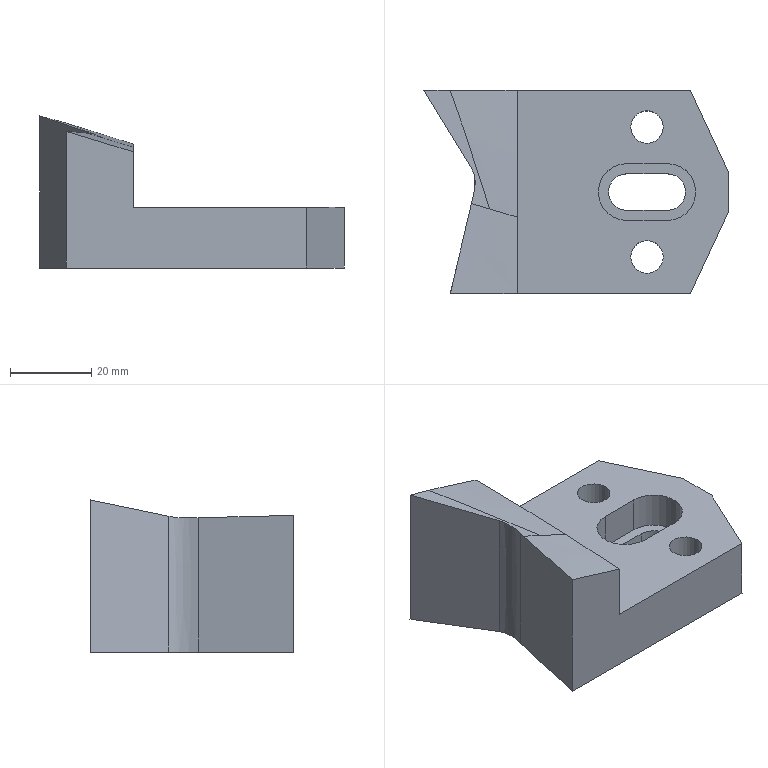Part | NX | features solid 2 | 1 solid | 25 faces | box 75.01 x 50.001 x 37.465 mm | volume 54539 mm3 | plane 13 | cylinder 6 | spline 6 | commonest cylinder face diameters 8 x2 9 x2 14 x2
STEP:
#1=CARTESIAN_POINT('',(745.,-33.,-80.));
#2=VERTEX_POINT('',#1);
#3=CARTESIAN_POINT('',(745.,-33.,-89.));
#4=VERTEX_POINT('',#3);
#5=CARTESIAN_POINT('',(745.,-33.,-90.));
#6=DIRECTION('',(0.000000502,-0.000000149,-1.));
#7=VECTOR('',#6,1000.);
#8=LINE('',#5,#7);
#9=EDGE_CURVE('',#2,#4,#8,.T.);
#10=ORIENTED_EDGE('',*,*,#9,.T.);
#11=CARTESIAN_POINT('',(745.,-47.,-89.));
#12=VERTEX_POINT('',#11);
#13=CARTESIAN_POINT('',(745.,-40.,-89.));
#14=DIRECTION('',(0.000000502,-0.000000149,-1.));
#15=DIRECTION('',(1.,0.,0.000000502));
#16=AXIS2_PLACEMENT_3D('',#13,#14,#15);
#17=CIRCLE('',#16,7.);
#18=EDGE_CURVE('',#4,#12,#17,.T.);
#19=ORIENTED_EDGE('',*,*,#18,.T.);
#20=CARTESIAN_POINT('',(745.,-47.,-80.));
#21=VERTEX_POINT('',#20);
#22=CARTESIAN_POINT('',(745.,-47.,-90.));
#23=DIRECTION('',(-0.000000502,0.000000149,1.));
#24=VECTOR('',#23,1000.);
#25=LINE('',#22,#24);
#26=EDGE_CURVE('',#21,#12,#25,.F.);
#27=ORIENTED_EDGE('',*,*,#26,.F.);
#28=CARTESIAN_POINT('',(745.,-40.,-80.));
#29=DIRECTION('',(-0.000000502,0.000000149,1.));
#30=DIRECTION('',(1.,0.,0.000000502));
#31=AXIS2_PLACEMENT_3D('',#28,#29,#30);
#32=CIRCLE('',#31,7.);
#33=EDGE_CURVE('',#21,#2,#32,.T.);
#34=ORIENTED_EDGE('',*,*,#33,.T.);
#35=EDGE_LOOP('',(#10,#19,#27,#34));
#36=FACE_BOUND('',#35,.T.);
#37=CARTESIAN_POINT('',(745.,-40.,-90.));
#38=DIRECTION('',(0.000000502,-0.000000149,-1.));
#39=DIRECTION('',(0.000001668,-1.,0.000000149));
#40=AXIS2_PLACEMENT_3D('',#37,#38,#39);
#41=CYLINDRICAL_SURFACE('',#40,7.);
#42=ADVANCED_FACE('',(#36),#41,.F.);
#43=ORIENTED_EDGE('',*,*,#26,.T.);
#44=CARTESIAN_POINT('',(735.,-47.,-89.));
#45=VERTEX_POINT('',#44);
#46=CARTESIAN_POINT('',(745.,-47.,-89.));
#47=DIRECTION('',(-1.,-0.000001668,-0.000000502));
#48=VECTOR('',#47,1000.);
#49=LINE('',#46,#48);
#50=EDGE_CURVE('',#12,#45,#49,.T.);
#51=ORIENTED_EDGE('',*,*,#50,.T.);
#52=CARTESIAN_POINT('',(735.,-47.,-80.));
#53=VERTEX_POINT('',#52);
#54=CARTESIAN_POINT('',(735.,-47.,-90.));
#55=DIRECTION('',(0.000000502,-0.000000149,-1.));
#56=VECTOR('',#55,1000.);
#57=LINE('',#54,#56);
#58=EDGE_CURVE('',#53,#45,#57,.T.);
#59=ORIENTED_EDGE('',*,*,#58,.F.);
#60=CARTESIAN_POINT('',(735.,-47.,-80.));
#61=DIRECTION('',(1.,0.000001668,0.000000502));
#62=VECTOR('',#61,1000.);
#63=LINE('',#60,#62);
#64=EDGE_CURVE('',#53,#21,#63,.T.);
#65=ORIENTED_EDGE('',*,*,#64,.T.);
#66=EDGE_LOOP('',(#43,#51,#59,#65));
#67=FACE_BOUND('',#66,.T.);
#68=CARTESIAN_POINT('',(735.,-47.,-90.));
#69=DIRECTION('',(-0.000001668,1.,-0.000000149));
#70=DIRECTION('',(-1.,-0.000001668,-0.000000502));
#71=AXIS2_PLACEMENT_3D('',#68,#69,#70);
#72=PLANE('',#71);
#73=ADVANCED_FACE('',(#67),#72,.T.);
#74=CARTESIAN_POINT('',(735.,-33.,-89.));
#75=VERTEX_POINT('',#74);
#76=CARTESIAN_POINT('',(735.,-40.,-89.));
#77=DIRECTION('',(-0.000000502,0.000000149,1.));
#78=DIRECTION('',(1.,0.,0.000000502));
#79=AXIS2_PLACEMENT_3D('',#76,#77,#78);
#80=CIRCLE('',#79,7.);
#81=EDGE_CURVE('',#75,#45,#80,.T.);
#82=ORIENTED_EDGE('',*,*,#81,.F.);
#83=CARTESIAN_POINT('',(735.,-33.,-80.));
#84=VERTEX_POINT('',#83);
#85=CARTESIAN_POINT('',(735.,-33.,-90.));
#86=DIRECTION('',(-0.000000502,0.000000149,1.));
#87=VECTOR('',#86,1000.);
#88=LINE('',#85,#87);
#89=EDGE_CURVE('',#84,#75,#88,.F.);
#90=ORIENTED_EDGE('',*,*,#89,.F.);
#91=CARTESIAN_POINT('',(735.,-40.,-80.));
#92=DIRECTION('',(-0.000000502,0.000000149,1.));
#93=DIRECTION('',(1.,0.,0.000000502));
#94=AXIS2_PLACEMENT_3D('',#91,#92,#93);
#95=CIRCLE('',#94,7.);
#96=EDGE_CURVE('',#53,#84,#95,.F.);
#97=ORIENTED_EDGE('',*,*,#96,.F.);
#98=ORIENTED_EDGE('',*,*,#58,.T.);
#99=EDGE_LOOP('',(#82,#90,#97,#98));
#100=FACE_BOUND('',#99,.T.);
#101=CARTESIAN_POINT('',(735.,-40.,-90.));
#102=DIRECTION('',(0.000000502,-0.000000149,-1.));
#103=DIRECTION('',(0.000001668,-1.,0.000000149));
#104=AXIS2_PLACEMENT_3D('',#101,#102,#103);
#105=CYLINDRICAL_SURFACE('',#104,7.);
#106=ADVANCED_FACE('',(#100),#105,.F.);
#107=CARTESIAN_POINT('',(745.,-33.,-89.));
#108=DIRECTION('',(-1.,-0.000001668,-0.000000502));
#109=VECTOR('',#108,1000.);
#110=LINE('',#107,#109);
#111=EDGE_CURVE('',#4,#75,#110,.T.);
#112=ORIENTED_EDGE('',*,*,#111,.F.);
#113=ORIENTED_EDGE('',*,*,#9,.F.);
#114=CARTESIAN_POINT('',(735.,-33.,-80.));
#115=DIRECTION('',(1.,0.000001668,0.000000502));
#116=VECTOR('',#115,1000.);
#117=LINE('',#114,#116);
#118=EDGE_CURVE('',#84,#2,#117,.T.);
#119=ORIENTED_EDGE('',*,*,#118,.F.);
#120=ORIENTED_EDGE('',*,*,#89,.T.);
#121=EDGE_LOOP('',(#112,#113,#119,#120));
#122=FACE_BOUND('',#121,.T.);
#123=CARTESIAN_POINT('',(735.,-33.,-90.));
#124=DIRECTION('',(-0.000001668,1.,-0.000000149));
#125=DIRECTION('',(-1.,-0.000001668,-0.000000502));
#126=AXIS2_PLACEMENT_3D('',#123,#124,#125);
#127=PLANE('',#126);
#128=ADVANCED_FACE('',(#122),#127,.F.);
#129=CARTESIAN_POINT('',(684.99,-15.,-95.));
#130=VERTEX_POINT('',#129);
#131=CARTESIAN_POINT('',(750.674,-15.,-95.));
#132=VERTEX_POINT('',#131);
#133=CARTESIAN_POINT('',(708.,-15.,-95.));
#134=DIRECTION('',(1.,0.000001668,0.000000502));
#135=VECTOR('',#134,1000.);
#136=LINE('',#133,#135);
#137=EDGE_CURVE('',#130,#132,#136,.T.);
#138=ORIENTED_EDGE('',*,*,#137,.T.);
#139=CARTESIAN_POINT('',(760.,-35.,-95.));
#140=VERTEX_POINT('',#139);
#141=CARTESIAN_POINT('',(750.674,-15.,-95.));
#142=DIRECTION('',(0.4226,-0.9063,0.000000347));
#143=VECTOR('',#142,1000.);
#144=LINE('',#141,#143);
#145=EDGE_CURVE('',#132,#140,#144,.T.);
#146=ORIENTED_EDGE('',*,*,#145,.T.);
#147=CARTESIAN_POINT('',(760.,-45.,-95.));
#148=VERTEX_POINT('',#147);
#149=CARTESIAN_POINT('',(760.,-45.,-95.));
#150=DIRECTION('',(-0.000001668,1.,-0.000000149));
#151=VECTOR('',#150,1000.);
#152=LINE('',#149,#151);
#153=EDGE_CURVE('',#148,#140,#152,.T.);
#154=ORIENTED_EDGE('',*,*,#153,.F.);
#155=CARTESIAN_POINT('',(750.674,-65.,-95.));
#156=VERTEX_POINT('',#155);
#157=CARTESIAN_POINT('',(750.674,-65.,-95.));
#158=DIRECTION('',(0.4226,0.9063,0.000000077));
#159=VECTOR('',#158,1000.);
#160=LINE('',#157,#159);
#161=EDGE_CURVE('',#156,#148,#160,.T.);
#162=ORIENTED_EDGE('',*,*,#161,.F.);
#163=CARTESIAN_POINT('',(691.52,-65.,-95.));
#164=VERTEX_POINT('',#163);
#165=CARTESIAN_POINT('',(700.,-65.,-95.));
#166=DIRECTION('',(1.,0.000001668,0.000000502));
#167=VECTOR('',#166,1000.);
#168=LINE('',#165,#167);
#169=EDGE_CURVE('',#164,#156,#168,.T.);
#170=ORIENTED_EDGE('',*,*,#169,.F.);
#171=CARTESIAN_POINT('',(697.072,-41.482,-95.));
#172=VERTEX_POINT('',#171);
#173=CARTESIAN_POINT('',(697.072,-41.482,-95.));
#174=CARTESIAN_POINT('',(695.176,-49.311,-95.));
#175=CARTESIAN_POINT('',(693.322,-57.15,-95.));
#176=CARTESIAN_POINT('',(691.52,-65.,-95.));
#177=B_SPLINE_CURVE_WITH_KNOTS('',3,(#173,#174,#175,#176),.UNSPECIFIED.,.F.,.F.,(4,4),(0.09346,0.1176),.UNSPECIFIED.);
#178=EDGE_CURVE('',#172,#164,#177,.T.);
#179=ORIENTED_EDGE('',*,*,#178,.F.);
#180=CARTESIAN_POINT('',(696.802,-34.28,-95.));
#181=VERTEX_POINT('',#180);
#182=CARTESIAN_POINT('',(696.802,-34.28,-95.));
#183=CARTESIAN_POINT('',(697.437,-35.339,-95.));
#184=CARTESIAN_POINT('',(697.892,-37.838,-95.));
#185=CARTESIAN_POINT('',(697.361,-40.28,-95.));
#186=CARTESIAN_POINT('',(697.072,-41.483,-95.));
#187=B_SPLINE_CURVE_WITH_KNOTS('',3,(#182,#183,#184,#185,#186),.UNSPECIFIED.,.F.,.F.,(4,1,4),(0.01374,0.01744,0.02115),.UNSPECIFIED.);
#188=EDGE_CURVE('',#172,#181,#187,.F.);
#189=ORIENTED_EDGE('',*,*,#188,.T.);
#190=CARTESIAN_POINT('',(684.99,-15.,-95.));
#191=CARTESIAN_POINT('',(688.941,-21.418,-95.));
#192=CARTESIAN_POINT('',(692.88,-27.844,-95.));
#193=CARTESIAN_POINT('',(696.802,-34.279,-95.));
#194=B_SPLINE_CURVE_WITH_KNOTS('',3,(#190,#191,#192,#193),.UNSPECIFIED.,.F.,.F.,(4,4),(0.,0.02261),.UNSPECIFIED.);
#195=EDGE_CURVE('',#130,#181,#194,.T.);
#196=ORIENTED_EDGE('',*,*,#195,.F.);
#197=EDGE_LOOP('',(#138,#146,#154,#162,#170,#179,#189,#196));
#198=FACE_BOUND('',#197,.T.);
#199=CARTESIAN_POINT('',(744.,-24.,-95.));
#200=VERTEX_POINT('',#199);
#201=CARTESIAN_POINT('',(740.,-24.,-95.));
#202=DIRECTION('',(-0.000000502,0.000000149,1.));
#203=DIRECTION('',(1.,0.,0.000000502));
#204=AXIS2_PLACEMENT_3D('',#201,#202,#203);
#205=CIRCLE('',#204,4.);
#206=EDGE_CURVE('',#200,#200,#205,.F.);
#207=ORIENTED_EDGE('',*,*,#206,.F.);
#208=EDGE_LOOP('',(#207));
#209=FACE_BOUND('',#208,.T.);
#210=CARTESIAN_POINT('',(744.,-56.,-95.));
#211=VERTEX_POINT('',#210);
#212=CARTESIAN_POINT('',(740.,-56.,-95.));
#213=DIRECTION('',(-0.000000502,0.000000149,1.));
#214=DIRECTION('',(1.,0.,0.000000502));
#215=AXIS2_PLACEMENT_3D('',#212,#213,#214);
#216=CIRCLE('',#215,4.);
#217=EDGE_CURVE('',#211,#211,#216,.F.);
#218=ORIENTED_EDGE('',*,*,#217,.F.);
#219=EDGE_LOOP('',(#218));
#220=FACE_BOUND('',#219,.T.);
#221=CARTESIAN_POINT('',(735.,-35.5,-95.));
#222=VERTEX_POINT('',#221);
#223=CARTESIAN_POINT('',(735.,-44.5,-95.));
#224=VERTEX_POINT('',#223);
#225=CARTESIAN_POINT('',(735.,-40.,-95.));
#226=DIRECTION('',(-0.000000502,0.000000149,1.));
#227=DIRECTION('',(1.,0.,0.000000502));
#228=AXIS2_PLACEMENT_3D('',#225,#226,#227);
#229=CIRCLE('',#228,4.5);
#230=EDGE_CURVE('',#222,#224,#229,.T.);
#231=ORIENTED_EDGE('',*,*,#230,.T.);
#232=CARTESIAN_POINT('',(745.,-44.5,-95.));
#233=VERTEX_POINT('',#232);
#234=CARTESIAN_POINT('',(735.,-44.5,-95.));
#235=DIRECTION('',(1.,0.000001668,0.000000502));
#236=VECTOR('',#235,1000.);
#237=LINE('',#234,#236);
#238=EDGE_CURVE('',#224,#233,#237,.T.);
#239=ORIENTED_EDGE('',*,*,#238,.T.);
#240=CARTESIAN_POINT('',(745.,-35.5,-95.));
#241=VERTEX_POINT('',#240);
#242=CARTESIAN_POINT('',(745.,-40.,-95.));
#243=DIRECTION('',(-0.000000502,0.000000149,1.));
#244=DIRECTION('',(1.,0.,0.000000502));
#245=AXIS2_PLACEMENT_3D('',#242,#243,#244);
#246=CIRCLE('',#245,4.5);
#247=EDGE_CURVE('',#233,#241,#246,.T.);
#248=ORIENTED_EDGE('',*,*,#247,.T.);
#249=CARTESIAN_POINT('',(735.,-35.5,-95.));
#250=DIRECTION('',(1.,0.000001668,0.000000502));
#251=VECTOR('',#250,1000.);
#252=LINE('',#249,#251);
#253=EDGE_CURVE('',#222,#241,#252,.T.);
#254=ORIENTED_EDGE('',*,*,#253,.F.);
#255=EDGE_LOOP('',(#231,#239,#248,#254));
#256=FACE_BOUND('',#255,.T.);
#257=CARTESIAN_POINT('',(700.,-15.,-95.));
#258=DIRECTION('',(0.000000502,-0.000000149,-1.));
#259=DIRECTION('',(0.000001668,-1.,0.000000149));
#260=AXIS2_PLACEMENT_3D('',#257,#258,#259);
#261=PLANE('',#260);
#262=ADVANCED_FACE('',(#198,#209,#220,#256),#261,.T.);
#263=CARTESIAN_POINT('',(691.497,-15.,-59.317));
#264=VERTEX_POINT('',#263);
#265=CARTESIAN_POINT('',(684.99,-15.,-57.535));
#266=VERTEX_POINT('',#265);
#267=CARTESIAN_POINT('',(691.486,-15.,-59.357));
#268=CARTESIAN_POINT('',(689.323,-15.,-58.741));
#269=CARTESIAN_POINT('',(687.16,-15.,-58.125));
#270=CARTESIAN_POINT('',(684.99,-15.,-57.535));
#271=B_SPLINE_CURVE_WITH_KNOTS('',3,(#267,#268,#269,#270),.UNSPECIFIED.,.F.,.F.,(4,4),(0.04155,0.0483),.UNSPECIFIED.);
#272=EDGE_CURVE('',#264,#266,#271,.T.);
#273=ORIENTED_EDGE('',*,*,#272,.F.);
#274=CARTESIAN_POINT('',(708.,-15.,-64.483));
#275=VERTEX_POINT('',#274);
#276=CARTESIAN_POINT('',(708.,-15.,-64.483));
#277=CARTESIAN_POINT('',(702.469,-15.,-62.856));
#278=CARTESIAN_POINT('',(697.041,-15.,-60.901));
#279=CARTESIAN_POINT('',(691.497,-15.,-59.317));
#280=B_SPLINE_CURVE_WITH_KNOTS('',3,(#276,#277,#278,#279),.UNSPECIFIED.,.F.,.F.,(4,4),(0.,0.01729),.UNSPECIFIED.);
#281=EDGE_CURVE('',#275,#264,#280,.T.);
#282=ORIENTED_EDGE('',*,*,#281,.F.);
#283=CARTESIAN_POINT('',(708.,-15.,-80.));
#284=VERTEX_POINT('',#283);
#285=CARTESIAN_POINT('',(708.,-15.,-105.));
#286=DIRECTION('',(-0.000000502,0.000000149,1.));
#287=VECTOR('',#286,1000.);
#288=LINE('',#285,#287);
#289=EDGE_CURVE('',#275,#284,#288,.F.);
#290=ORIENTED_EDGE('',*,*,#289,.T.);
#291=CARTESIAN_POINT('',(750.674,-15.,-80.));
#292=VERTEX_POINT('',#291);
#293=CARTESIAN_POINT('',(708.,-15.,-80.));
#294=DIRECTION('',(1.,0.000001668,0.000000502));
#295=VECTOR('',#294,1000.);
#296=LINE('',#293,#295);
#297=EDGE_CURVE('',#284,#292,#296,.T.);
#298=ORIENTED_EDGE('',*,*,#297,.T.);
#299=CARTESIAN_POINT('',(750.674,-15.,-90.));
#300=DIRECTION('',(0.000000502,-0.000000149,-1.));
#301=VECTOR('',#300,1000.);
#302=LINE('',#299,#301);
#303=EDGE_CURVE('',#292,#132,#302,.T.);
#304=ORIENTED_EDGE('',*,*,#303,.T.);
#305=ORIENTED_EDGE('',*,*,#137,.F.);
#306=CARTESIAN_POINT('',(684.99,-15.,-57.535));
#307=CARTESIAN_POINT('',(684.99,-15.,-70.023));
#308=CARTESIAN_POINT('',(684.99,-15.,-82.512));
#309=CARTESIAN_POINT('',(684.99,-15.,-95.));
#310=B_SPLINE_CURVE_WITH_KNOTS('',3,(#306,#307,#308,#309),.UNSPECIFIED.,.F.,.F.,(4,4),(0.00214,0.03961),.UNSPECIFIED.);
#311=EDGE_CURVE('',#266,#130,#310,.T.);
#312=ORIENTED_EDGE('',*,*,#311,.F.);
#313=EDGE_LOOP('',(#273,#282,#290,#298,#304,#305,#312));
#314=FACE_BOUND('',#313,.T.);
#315=CARTESIAN_POINT('',(708.,-15.,-90.));
#316=DIRECTION('',(-0.000001668,1.,-0.000000149));
#317=DIRECTION('',(-1.,-0.000001668,-0.000000502));
#318=AXIS2_PLACEMENT_3D('',#315,#316,#317);
#319=PLANE('',#318);
#320=ADVANCED_FACE('',(#314),#319,.T.);
#321=CARTESIAN_POINT('',(691.535,-65.,-61.337));
#322=VERTEX_POINT('',#321);
#323=CARTESIAN_POINT('',(691.535,-65.,-61.337));
#324=CARTESIAN_POINT('',(691.53,-65.,-72.558));
#325=CARTESIAN_POINT('',(691.525,-65.,-83.779));
#326=CARTESIAN_POINT('',(691.52,-65.,-95.));
#327=B_SPLINE_CURVE_WITH_KNOTS('',3,(#323,#324,#325,#326),.UNSPECIFIED.,.F.,.F.,(4,4),(0.002194,0.03586),.UNSPECIFIED.);
#328=EDGE_CURVE('',#322,#164,#327,.T.);
#329=ORIENTED_EDGE('',*,*,#328,.T.);
#330=ORIENTED_EDGE('',*,*,#169,.T.);
#331=CARTESIAN_POINT('',(750.674,-65.,-80.));
#332=VERTEX_POINT('',#331);
#333=CARTESIAN_POINT('',(750.674,-65.,-90.));
#334=DIRECTION('',(0.000000502,-0.000000149,-1.));
#335=VECTOR('',#334,1000.);
#336=LINE('',#333,#335);
#337=EDGE_CURVE('',#332,#156,#336,.T.);
#338=ORIENTED_EDGE('',*,*,#337,.F.);
#339=CARTESIAN_POINT('',(708.,-65.,-80.));
#340=VERTEX_POINT('',#339);
#341=CARTESIAN_POINT('',(700.,-65.,-80.));
#342=DIRECTION('',(1.,0.000001668,0.000000502));
#343=VECTOR('',#342,1000.);
#344=LINE('',#341,#343);
#345=EDGE_CURVE('',#340,#332,#344,.T.);
#346=ORIENTED_EDGE('',*,*,#345,.F.);
#347=CARTESIAN_POINT('',(708.,-65.,-66.363));
#348=VERTEX_POINT('',#347);
#349=CARTESIAN_POINT('',(708.,-65.,-105.));
#350=DIRECTION('',(-0.000000502,0.000000149,1.));
#351=VECTOR('',#350,1000.);
#352=LINE('',#349,#351);
#353=EDGE_CURVE('',#348,#340,#352,.F.);
#354=ORIENTED_EDGE('',*,*,#353,.F.);
#355=CARTESIAN_POINT('',(691.535,-65.,-61.337));
#356=CARTESIAN_POINT('',(697.046,-65.,-62.922));
#357=CARTESIAN_POINT('',(702.528,-65.,-64.628));
#358=CARTESIAN_POINT('',(708.,-65.,-66.363));
#359=B_SPLINE_CURVE_WITH_KNOTS('',3,(#355,#356,#357,#358),.UNSPECIFIED.,.F.,.F.,(4,4),(0.0434,0.0606),.UNSPECIFIED.);
#360=EDGE_CURVE('',#322,#348,#359,.T.);
#361=ORIENTED_EDGE('',*,*,#360,.F.);
#362=EDGE_LOOP('',(#329,#330,#338,#346,#354,#361));
#363=FACE_BOUND('',#362,.T.);
#364=CARTESIAN_POINT('',(700.,-65.,-90.));
#365=DIRECTION('',(-0.000001668,1.,-0.000000149));
#366=DIRECTION('',(0.000000502,-0.000000149,-1.));
#367=AXIS2_PLACEMENT_3D('',#364,#365,#366);
#368=PLANE('',#367);
#369=ADVANCED_FACE('',(#363),#368,.F.);
#370=CARTESIAN_POINT('',(696.733,-42.883,-61.871));
#371=VERTEX_POINT('',#370);
#372=CARTESIAN_POINT('',(696.733,-42.883,-61.871));
#373=CARTESIAN_POINT('',(694.956,-50.244,-61.658));
#374=CARTESIAN_POINT('',(693.223,-57.617,-61.47));
#375=CARTESIAN_POINT('',(691.535,-65.,-61.337));
#376=B_SPLINE_CURVE_WITH_KNOTS('',3,(#372,#373,#374,#375),.UNSPECIFIED.,.F.,.F.,(4,4),(0.1439,0.1667),.UNSPECIFIED.);
#377=EDGE_CURVE('',#371,#322,#376,.T.);
#378=ORIENTED_EDGE('',*,*,#377,.T.);
#379=ORIENTED_EDGE('',*,*,#360,.T.);
#380=CARTESIAN_POINT('',(708.,-46.209,-65.274));
#381=VERTEX_POINT('',#380);
#382=CARTESIAN_POINT('',(708.,-65.,-66.363));
#383=CARTESIAN_POINT('',(708.,-63.434,-66.267));
#384=CARTESIAN_POINT('',(708.,-61.092,-66.12));
#385=CARTESIAN_POINT('',(708.,-58.339,-65.945));
#386=CARTESIAN_POINT('',(708.,-56.795,-65.847));
#387=CARTESIAN_POINT('',(708.,-55.553,-65.766));
#388=CARTESIAN_POINT('',(708.,-54.635,-65.708));
#389=CARTESIAN_POINT('',(708.,-53.211,-65.623));
#390=CARTESIAN_POINT('',(708.,-50.605,-65.479));
#391=CARTESIAN_POINT('',(708.,-48.045,-65.356));
#392=CARTESIAN_POINT('',(708.,-46.209,-65.274));
#393=B_SPLINE_CURVE_WITH_KNOTS('',3,(#382,#383,#384,#385,#386,#387,#388,#389,#390,#391,#392),.UNSPECIFIED.,.F.,.F.,(4,1,1,1,1,1,1,1,4),(0.,0.25,0.375,0.4375,0.5,0.5625,0.625,0.75,1.),.UNSPECIFIED.);
#394=EDGE_CURVE('',#381,#348,#393,.F.);
#395=ORIENTED_EDGE('',*,*,#394,.F.);
#396=CARTESIAN_POINT('',(701.201,-44.201,-63.22));
#397=VERTEX_POINT('',#396);
#398=CARTESIAN_POINT('',(701.2,-44.202,-63.22));
#399=CARTESIAN_POINT('',(703.467,-44.871,-63.905));
#400=CARTESIAN_POINT('',(705.733,-45.54,-64.589));
#401=CARTESIAN_POINT('',(708.,-46.209,-65.274));
#402=B_SPLINE_CURVE_WITH_KNOTS('',3,(#398,#399,#400,#401),.UNSPECIFIED.,.F.,.F.,(4,4),(0.4767,0.7872),.UNSPECIFIED.);
#403=EDGE_CURVE('',#397,#381,#402,.T.);
#404=ORIENTED_EDGE('',*,*,#403,.F.);
#405=CARTESIAN_POINT('',(696.733,-42.883,-61.871));
#406=CARTESIAN_POINT('',(698.222,-43.323,-62.321));
#407=CARTESIAN_POINT('',(699.711,-43.762,-62.77));
#408=CARTESIAN_POINT('',(701.2,-44.202,-63.22));
#409=B_SPLINE_CURVE_WITH_KNOTS('',3,(#405,#406,#407,#408),.UNSPECIFIED.,.F.,.F.,(4,4),(0.2727,0.4767),.UNSPECIFIED.);
#410=EDGE_CURVE('',#371,#397,#409,.T.);
#411=ORIENTED_EDGE('',*,*,#410,.F.);
#412=EDGE_LOOP('',(#378,#379,#395,#404,#411));
#413=FACE_BOUND('',#412,.T.);
#414=CARTESIAN_POINT('',(707.217,-68.842,-66.332));
#415=CARTESIAN_POINT('',(708.034,-65.269,-66.411));
#416=CARTESIAN_POINT('',(709.678,-58.129,-66.434));
#417=CARTESIAN_POINT('',(711.425,-51.027,-66.483));
#418=CARTESIAN_POINT('',(712.345,-47.491,-66.586));
#419=CARTESIAN_POINT('',(701.97,-67.603,-64.574));
#420=CARTESIAN_POINT('',(702.795,-63.984,-64.655));
#421=CARTESIAN_POINT('',(704.448,-56.747,-64.764));
#422=CARTESIAN_POINT('',(706.192,-49.538,-64.898));
#423=CARTESIAN_POINT('',(707.11,-45.946,-65.005));
#424=CARTESIAN_POINT('',(696.701,-66.359,-62.886));
#425=CARTESIAN_POINT('',(697.536,-62.692,-62.963));
#426=CARTESIAN_POINT('',(699.208,-55.36,-63.123));
#427=CARTESIAN_POINT('',(700.959,-48.048,-63.314));
#428=CARTESIAN_POINT('',(701.875,-44.401,-63.424));
#429=CARTESIAN_POINT('',(691.402,-65.109,-61.304));
#430=CARTESIAN_POINT('',(692.251,-61.394,-61.371));
#431=CARTESIAN_POINT('',(693.957,-53.966,-61.527));
#432=CARTESIAN_POINT('',(695.727,-46.555,-61.73));
#433=CARTESIAN_POINT('',(696.64,-42.856,-61.843));
#434=B_SPLINE_SURFACE_WITH_KNOTS('',3,3,((#414,#415,#416,#417,#418),(#419,#420,#421,#422,#423),(#424,#425,#426,#427,#428),(#429,#430,#431,#432,#433)),.UNSPECIFIED.,.F.,.F.,.F.,(4,4),(4,1,4),(0.0881,0.7516),(0.04208,0.521,1.),.UNSPECIFIED.);
#435=ADVANCED_FACE('',(#413),#434,.F.);
#436=CARTESIAN_POINT('',(696.802,-34.279,-61.549));
#437=VERTEX_POINT('',#436);
#438=CARTESIAN_POINT('',(697.072,-41.482,-61.912));
#439=VERTEX_POINT('',#438);
#440=CARTESIAN_POINT('',(696.802,-34.279,-61.549));
#441=CARTESIAN_POINT('',(697.43,-35.326,-61.77));
#442=CARTESIAN_POINT('',(697.897,-37.829,-62.003));
#443=CARTESIAN_POINT('',(697.362,-40.276,-61.947));
#444=CARTESIAN_POINT('',(697.072,-41.483,-61.912));
#445=B_SPLINE_CURVE_WITH_KNOTS('',3,(#440,#441,#442,#443,#444),.UNSPECIFIED.,.F.,.F.,(4,1,4),(0.01176,0.01548,0.0192),.UNSPECIFIED.);
#446=EDGE_CURVE('',#437,#439,#445,.T.);
#447=ORIENTED_EDGE('',*,*,#446,.T.);
#448=CARTESIAN_POINT('',(696.733,-42.883,-61.871));
#449=CARTESIAN_POINT('',(696.846,-42.416,-61.885));
#450=CARTESIAN_POINT('',(696.959,-41.949,-61.898));
#451=CARTESIAN_POINT('',(697.072,-41.482,-61.912));
#452=B_SPLINE_CURVE_WITH_KNOTS('',3,(#448,#449,#450,#451),.UNSPECIFIED.,.F.,.F.,(4,4),(0.,0.001442),.UNSPECIFIED.);
#453=EDGE_CURVE('',#371,#439,#452,.T.);
#454=ORIENTED_EDGE('',*,*,#453,.F.);
#455=ORIENTED_EDGE('',*,*,#410,.T.);
#456=CARTESIAN_POINT('',(695.108,-25.285,-60.731));
#457=VERTEX_POINT('',#456);
#458=CARTESIAN_POINT('',(701.201,-44.2,-63.22));
#459=CARTESIAN_POINT('',(699.21,-38.,-62.382));
#460=CARTESIAN_POINT('',(697.18,-31.694,-61.551));
#461=CARTESIAN_POINT('',(695.109,-25.284,-60.732));
#462=B_SPLINE_CURVE_WITH_KNOTS('',3,(#458,#459,#460,#461),.UNSPECIFIED.,.F.,.F.,(4,4),(0.,0.2626),.UNSPECIFIED.);
#463=EDGE_CURVE('',#397,#457,#462,.T.);
#464=ORIENTED_EDGE('',*,*,#463,.T.);
#465=CARTESIAN_POINT('',(695.108,-25.284,-60.732));
#466=CARTESIAN_POINT('',(693.918,-21.621,-60.262));
#467=CARTESIAN_POINT('',(692.708,-18.186,-59.804));
#468=CARTESIAN_POINT('',(691.48,-14.985,-59.355));
#469=B_SPLINE_CURVE_WITH_KNOTS('',3,(#465,#466,#467,#468),.UNSPECIFIED.,.F.,.F.,(4,4),(0.01082,0.3147),.UNSPECIFIED.);
#470=EDGE_CURVE('',#457,#264,#469,.T.);
#471=ORIENTED_EDGE('',*,*,#470,.T.);
#472=ORIENTED_EDGE('',*,*,#272,.T.);
#473=CARTESIAN_POINT('',(696.802,-34.279,-61.549));
#474=CARTESIAN_POINT('',(692.883,-27.849,-60.173));
#475=CARTESIAN_POINT('',(688.946,-21.425,-58.809));
#476=CARTESIAN_POINT('',(684.99,-15.,-57.535));
#477=B_SPLINE_CURVE_WITH_KNOTS('',3,(#473,#474,#475,#476),.UNSPECIFIED.,.F.,.F.,(4,4),(0.1292,0.1521),.UNSPECIFIED.);
#478=EDGE_CURVE('',#437,#266,#477,.T.);
#479=ORIENTED_EDGE('',*,*,#478,.F.);
#480=EDGE_LOOP('',(#447,#454,#455,#464,#471,#472,#479));
#481=FACE_BOUND('',#480,.T.);
#482=CARTESIAN_POINT('',(701.297,-44.386,-63.256));
#483=CARTESIAN_POINT('',(696.609,-43.003,-61.851));
#484=CARTESIAN_POINT('',(691.903,-41.618,-60.391));
#485=CARTESIAN_POINT('',(687.233,-40.237,-59.041));
#486=CARTESIAN_POINT('',(700.592,-35.466,-62.673));
#487=CARTESIAN_POINT('',(695.858,-33.953,-61.261));
#488=CARTESIAN_POINT('',(691.106,-32.435,-59.794));
#489=CARTESIAN_POINT('',(686.391,-30.927,-58.438));
#490=CARTESIAN_POINT('',(699.871,-26.547,-62.126));
#491=CARTESIAN_POINT('',(695.091,-24.907,-60.71));
#492=CARTESIAN_POINT('',(690.294,-23.258,-59.239));
#493=CARTESIAN_POINT('',(685.532,-21.625,-57.879));
#494=CARTESIAN_POINT('',(699.134,-17.631,-61.617));
#495=CARTESIAN_POINT('',(694.308,-15.865,-60.199));
#496=CARTESIAN_POINT('',(689.465,-14.087,-58.725));
#497=CARTESIAN_POINT('',(684.657,-12.332,-57.363));
#498=B_SPLINE_SURFACE_WITH_KNOTS('',3,3,((#482,#483,#484,#485),(#486,#487,#488,#489),(#490,#491,#492,#493),(#494,#495,#496,#497)),.UNSPECIFIED.,.F.,.F.,.F.,(4,4),(4,4),(-0.0006687,0.1104),(0.1077,0.2017),.UNSPECIFIED.);
#499=ADVANCED_FACE('',(#481),#498,.T.);
#500=ORIENTED_EDGE('',*,*,#394,.T.);
#501=ORIENTED_EDGE('',*,*,#353,.T.);
#502=CARTESIAN_POINT('',(708.,-15.,-80.));
#503=DIRECTION('',(-0.000001668,1.,-0.000000149));
#504=VECTOR('',#503,1000.);
#505=LINE('',#502,#504);
#506=EDGE_CURVE('',#284,#340,#505,.F.);
#507=ORIENTED_EDGE('',*,*,#506,.F.);
#508=ORIENTED_EDGE('',*,*,#289,.F.);
#509=CARTESIAN_POINT('',(708.,-46.209,-65.274));
#510=CARTESIAN_POINT('',(708.,-36.298,-64.834));
#511=CARTESIAN_POINT('',(708.,-25.895,-64.57));
#512=CARTESIAN_POINT('',(708.,-15.,-64.483));
#513=B_SPLINE_CURVE_WITH_KNOTS('',3,(#509,#510,#511,#512),.UNSPECIFIED.,.F.,.F.,(4,4),(0.,1.),.UNSPECIFIED.);
#514=EDGE_CURVE('',#381,#275,#513,.T.);
#515=ORIENTED_EDGE('',*,*,#514,.F.);
#516=EDGE_LOOP('',(#500,#501,#507,#508,#515));
#517=FACE_BOUND('',#516,.T.);
#518=CARTESIAN_POINT('',(708.,-15.,-105.));
#519=DIRECTION('',(-1.,-0.000001668,-0.000000502));
#520=DIRECTION('',(0.000001668,-1.,0.000000149));
#521=AXIS2_PLACEMENT_3D('',#518,#519,#520);
#522=PLANE('',#521);
#523=ADVANCED_FACE('',(#517),#522,.F.);
#524=CARTESIAN_POINT('',(744.,-24.,-80.));
#525=VERTEX_POINT('',#524);
#526=CARTESIAN_POINT('',(740.,-24.,-80.));
#527=DIRECTION('',(-0.000000502,0.000000149,1.));
#528=DIRECTION('',(1.,0.,0.000000502));
#529=AXIS2_PLACEMENT_3D('',#526,#527,#528);
#530=CIRCLE('',#529,4.);
#531=EDGE_CURVE('',#525,#525,#530,.F.);
#532=ORIENTED_EDGE('',*,*,#531,.T.);
#533=EDGE_LOOP('',(#532));
#534=FACE_BOUND('',#533,.T.);
#535=CARTESIAN_POINT('',(744.,-56.,-80.));
#536=VERTEX_POINT('',#535);
#537=CARTESIAN_POINT('',(740.,-56.,-80.));
#538=DIRECTION('',(-0.000000502,0.000000149,1.));
#539=DIRECTION('',(1.,0.,0.000000502));
#540=AXIS2_PLACEMENT_3D('',#537,#538,#539);
#541=CIRCLE('',#540,4.);
#542=EDGE_CURVE('',#536,#536,#541,.F.);
#543=ORIENTED_EDGE('',*,*,#542,.T.);
#544=EDGE_LOOP('',(#543));
#545=FACE_BOUND('',#544,.T.);
#546=ORIENTED_EDGE('',*,*,#297,.F.);
#547=ORIENTED_EDGE('',*,*,#506,.T.);
#548=ORIENTED_EDGE('',*,*,#345,.T.);
#549=CARTESIAN_POINT('',(760.,-45.,-80.));
#550=VERTEX_POINT('',#549);
#551=CARTESIAN_POINT('',(750.674,-65.,-80.));
#552=DIRECTION('',(0.4226,0.9063,0.000000077));
#553=VECTOR('',#552,1000.);
#554=LINE('',#551,#553);
#555=EDGE_CURVE('',#332,#550,#554,.T.);
#556=ORIENTED_EDGE('',*,*,#555,.T.);
#557=CARTESIAN_POINT('',(760.,-35.,-80.));
#558=VERTEX_POINT('',#557);
#559=CARTESIAN_POINT('',(760.,-45.,-80.));
#560=DIRECTION('',(-0.000001668,1.,-0.000000149));
#561=VECTOR('',#560,1000.);
#562=LINE('',#559,#561);
#563=EDGE_CURVE('',#550,#558,#562,.T.);
#564=ORIENTED_EDGE('',*,*,#563,.T.);
#565=CARTESIAN_POINT('',(750.674,-15.,-80.));
#566=DIRECTION('',(0.4226,-0.9063,0.000000347));
#567=VECTOR('',#566,1000.);
#568=LINE('',#565,#567);
#569=EDGE_CURVE('',#292,#558,#568,.T.);
#570=ORIENTED_EDGE('',*,*,#569,.F.);
#571=EDGE_LOOP('',(#546,#547,#548,#556,#564,#570));
#572=FACE_BOUND('',#571,.T.);
#573=ORIENTED_EDGE('',*,*,#33,.F.);
#574=ORIENTED_EDGE('',*,*,#64,.F.);
#575=ORIENTED_EDGE('',*,*,#96,.T.);
#576=ORIENTED_EDGE('',*,*,#118,.T.);
#577=EDGE_LOOP('',(#573,#574,#575,#576));
#578=FACE_BOUND('',#577,.T.);
#579=CARTESIAN_POINT('',(700.,-15.,-80.));
#580=DIRECTION('',(0.000000502,-0.000000149,-1.));
#581=DIRECTION('',(0.000001668,-1.,0.000000149));
#582=AXIS2_PLACEMENT_3D('',#579,#580,#581);
#583=PLANE('',#582);
#584=ADVANCED_FACE('',(#534,#545,#572,#578),#583,.F.);
#585=ORIENTED_EDGE('',*,*,#145,.F.);
#586=ORIENTED_EDGE('',*,*,#303,.F.);
#587=ORIENTED_EDGE('',*,*,#569,.T.);
#588=CARTESIAN_POINT('',(760.,-35.,-90.));
#589=DIRECTION('',(0.000000502,-0.000000149,-1.));
#590=VECTOR('',#589,1000.);
#591=LINE('',#588,#590);
#592=EDGE_CURVE('',#558,#140,#591,.T.);
#593=ORIENTED_EDGE('',*,*,#592,.T.);
#594=EDGE_LOOP('',(#585,#586,#587,#593));
#595=FACE_BOUND('',#594,.T.);
#596=CARTESIAN_POINT('',(750.674,-15.,-90.));
#597=DIRECTION('',(0.9063,0.4226,0.000000392));
#598=DIRECTION('',(-0.4226,0.9063,-0.000000347));
#599=AXIS2_PLACEMENT_3D('',#596,#597,#598);
#600=PLANE('',#599);
#601=ADVANCED_FACE('',(#595),#600,.T.);
#602=ORIENTED_EDGE('',*,*,#153,.T.);
#603=ORIENTED_EDGE('',*,*,#592,.F.);
#604=ORIENTED_EDGE('',*,*,#563,.F.);
#605=CARTESIAN_POINT('',(760.,-45.,-90.));
#606=DIRECTION('',(0.000000502,-0.000000149,-1.));
#607=VECTOR('',#606,1000.);
#608=LINE('',#605,#607);
#609=EDGE_CURVE('',#550,#148,#608,.T.);
#610=ORIENTED_EDGE('',*,*,#609,.T.);
#611=EDGE_LOOP('',(#602,#603,#604,#610));
#612=FACE_BOUND('',#611,.T.);
#613=CARTESIAN_POINT('',(760.,-45.,-90.));
#614=DIRECTION('',(-1.,-0.000001668,-0.000000502));
#615=DIRECTION('',(-0.000000502,0.000000149,1.));
#616=AXIS2_PLACEMENT_3D('',#613,#614,#615);
#617=PLANE('',#616);
#618=ADVANCED_FACE('',(#612),#617,.F.);
#619=ORIENTED_EDGE('',*,*,#161,.T.);
#620=ORIENTED_EDGE('',*,*,#609,.F.);
#621=ORIENTED_EDGE('',*,*,#555,.F.);
#622=ORIENTED_EDGE('',*,*,#337,.T.);
#623=EDGE_LOOP('',(#619,#620,#621,#622));
#624=FACE_BOUND('',#623,.T.);
#625=CARTESIAN_POINT('',(750.674,-65.,-90.));
#626=DIRECTION('',(-0.9063,0.4226,-0.000000518));
#627=DIRECTION('',(-0.4226,-0.9063,-0.000000077));
#628=AXIS2_PLACEMENT_3D('',#625,#626,#627);
#629=PLANE('',#628);
#630=ADVANCED_FACE('',(#624),#629,.F.);
#631=ORIENTED_EDGE('',*,*,#217,.T.);
#632=EDGE_LOOP('',(#631));
#633=FACE_BOUND('',#632,.T.);
#634=ORIENTED_EDGE('',*,*,#542,.F.);
#635=EDGE_LOOP('',(#634));
#636=FACE_BOUND('',#635,.T.);
#637=CARTESIAN_POINT('',(740.,-56.,-90.));
#638=DIRECTION('',(0.000000502,-0.000000149,-1.));
#639=DIRECTION('',(0.000001668,-1.,0.000000149));
#640=AXIS2_PLACEMENT_3D('',#637,#638,#639);
#641=CYLINDRICAL_SURFACE('',#640,4.);
#642=ADVANCED_FACE('',(#633,#636),#641,.F.);
#643=ORIENTED_EDGE('',*,*,#206,.T.);
#644=EDGE_LOOP('',(#643));
#645=FACE_BOUND('',#644,.T.);
#646=ORIENTED_EDGE('',*,*,#531,.F.);
#647=EDGE_LOOP('',(#646));
#648=FACE_BOUND('',#647,.T.);
#649=CARTESIAN_POINT('',(740.,-24.,-90.));
#650=DIRECTION('',(0.000000502,-0.000000149,-1.));
#651=DIRECTION('',(0.000001668,-1.,0.000000149));
#652=AXIS2_PLACEMENT_3D('',#649,#650,#651);
#653=CYLINDRICAL_SURFACE('',#652,4.);
#654=ADVANCED_FACE('',(#645,#648),#653,.F.);
#655=ORIENTED_EDGE('',*,*,#281,.T.);
#656=ORIENTED_EDGE('',*,*,#470,.F.);
#657=ORIENTED_EDGE('',*,*,#463,.F.);
#658=ORIENTED_EDGE('',*,*,#403,.T.);
#659=ORIENTED_EDGE('',*,*,#514,.T.);
#660=EDGE_LOOP('',(#655,#656,#657,#658,#659));
#661=FACE_BOUND('',#660,.T.);
#662=CARTESIAN_POINT('',(691.426,-14.814,-59.291));
#663=CARTESIAN_POINT('',(694.129,-14.055,-60.04));
#664=CARTESIAN_POINT('',(699.482,-12.531,-61.765));
#665=CARTESIAN_POINT('',(704.844,-10.996,-63.534));
#666=CARTESIAN_POINT('',(707.557,-10.228,-64.327));
#667=CARTESIAN_POINT('',(692.516,-17.635,-59.687));
#668=CARTESIAN_POINT('',(695.107,-16.996,-60.4));
#669=CARTESIAN_POINT('',(700.243,-15.716,-62.026));
#670=CARTESIAN_POINT('',(705.387,-14.43,-63.703));
#671=CARTESIAN_POINT('',(707.986,-13.785,-64.463));
#672=CARTESIAN_POINT('',(694.238,-22.531,-60.387));
#673=CARTESIAN_POINT('',(696.639,-22.095,-61.063));
#674=CARTESIAN_POINT('',(701.417,-21.22,-62.526));
#675=CARTESIAN_POINT('',(706.203,-20.341,-64.007));
#676=CARTESIAN_POINT('',(708.613,-19.9,-64.701));
#677=CARTESIAN_POINT('',(697.406,-32.436,-61.642));
#678=CARTESIAN_POINT('',(699.423,-32.39,-62.217));
#679=CARTESIAN_POINT('',(703.45,-32.3,-63.399));
#680=CARTESIAN_POINT('',(707.481,-32.209,-64.589));
#681=CARTESIAN_POINT('',(709.5,-32.163,-65.173));
#682=CARTESIAN_POINT('',(699.675,-39.431,-62.577));
#683=CARTESIAN_POINT('',(701.364,-39.667,-63.076));
#684=CARTESIAN_POINT('',(704.744,-40.14,-64.068));
#685=CARTESIAN_POINT('',(708.123,-40.614,-65.055));
#686=CARTESIAN_POINT('',(709.813,-40.85,-65.55));
#687=CARTESIAN_POINT('',(701.257,-44.377,-63.244));
#688=CARTESIAN_POINT('',(702.691,-44.81,-63.678));
#689=CARTESIAN_POINT('',(705.557,-45.676,-64.545));
#690=CARTESIAN_POINT('',(708.424,-46.542,-65.411));
#691=CARTESIAN_POINT('',(709.858,-46.975,-65.845));
#692=B_SPLINE_SURFACE_WITH_KNOTS('',3,3,((#662,#663,#664,#665,#666),(#667,#668,#669,#670,#671),(#672,#673,#674,#675,#676),(#677,#678,#679,#680,#681),(#682,#683,#684,#685,#686),(#687,#688,#689,#690,#691)),.UNSPECIFIED.,.F.,.F.,.F.,(4,1,1,4),(4,1,4),(0.5877,0.7086,0.7951,1.002),(0.,0.4093,0.8186),.UNSPECIFIED.);
#693=ADVANCED_FACE('',(#661),#692,.T.);
#694=ORIENTED_EDGE('',*,*,#195,.T.);
#695=CARTESIAN_POINT('',(696.802,-34.279,-95.));
#696=CARTESIAN_POINT('',(696.802,-34.279,-83.85));
#697=CARTESIAN_POINT('',(696.802,-34.279,-72.7));
#698=CARTESIAN_POINT('',(696.802,-34.279,-61.549));
#699=B_SPLINE_CURVE_WITH_KNOTS('',3,(#695,#696,#697,#698),.UNSPECIFIED.,.F.,.F.,(4,4),(0.4121,0.5072),.UNSPECIFIED.);
#700=EDGE_CURVE('',#181,#437,#699,.T.);
#701=ORIENTED_EDGE('',*,*,#700,.T.);
#702=ORIENTED_EDGE('',*,*,#478,.T.);
#703=ORIENTED_EDGE('',*,*,#311,.T.);
#704=EDGE_LOOP('',(#694,#701,#702,#703));
#705=FACE_BOUND('',#704,.T.);
#706=CARTESIAN_POINT('',(684.919,-14.884,-57.288));
#707=CARTESIAN_POINT('',(684.919,-14.884,-95.203));
#708=CARTESIAN_POINT('',(688.901,-21.352,-58.516));
#709=CARTESIAN_POINT('',(688.901,-21.352,-96.431));
#710=CARTESIAN_POINT('',(692.864,-27.817,-59.82));
#711=CARTESIAN_POINT('',(692.864,-27.817,-97.734));
#712=CARTESIAN_POINT('',(696.826,-34.318,-61.207));
#713=CARTESIAN_POINT('',(696.826,-34.318,-99.122));
#714=CARTESIAN_POINT('',(696.849,-34.357,-61.215));
#715=CARTESIAN_POINT('',(696.849,-34.357,-99.13));
#716=CARTESIAN_POINT('',(696.873,-34.395,-61.224));
#717=CARTESIAN_POINT('',(696.873,-34.395,-99.138));
#718=B_SPLINE_SURFACE_WITH_KNOTS('',3,1,((#706,#707),(#708,#709),(#710,#711),(#712,#713),(#714,#715),(#716,#717)),.RULED_SURF.,.F.,.F.,.F.,(4,2,4),(2,2),(0.7699,0.8177,0.818),(0.4908,0.6041),.UNSPECIFIED.);
#719=ADVANCED_FACE('',(#705),#718,.F.);
#720=CARTESIAN_POINT('',(697.072,-41.483,-95.));
#721=CARTESIAN_POINT('',(697.072,-41.483,-83.971));
#722=CARTESIAN_POINT('',(697.072,-41.483,-72.941));
#723=CARTESIAN_POINT('',(697.072,-41.483,-61.912));
#724=B_SPLINE_CURVE_WITH_KNOTS('',3,(#720,#721,#722,#723),.UNSPECIFIED.,.F.,.F.,(4,4),(0.4082,0.5078),.UNSPECIFIED.);
#725=EDGE_CURVE('',#172,#439,#724,.T.);
#726=ORIENTED_EDGE('',*,*,#725,.T.);
#727=ORIENTED_EDGE('',*,*,#446,.F.);
#728=ORIENTED_EDGE('',*,*,#700,.F.);
#729=ORIENTED_EDGE('',*,*,#188,.F.);
#730=EDGE_LOOP('',(#726,#727,#728,#729));
#731=FACE_BOUND('',#730,.T.);
#732=CARTESIAN_POINT('',(697.062,-41.526,-61.575));
#733=CARTESIAN_POINT('',(697.062,-41.526,-72.783));
#734=CARTESIAN_POINT('',(697.062,-41.526,-83.99));
#735=CARTESIAN_POINT('',(697.062,-41.526,-95.198));
#736=CARTESIAN_POINT('',(697.065,-41.512,-61.576));
#737=CARTESIAN_POINT('',(697.065,-41.512,-72.783));
#738=CARTESIAN_POINT('',(697.065,-41.512,-83.991));
#739=CARTESIAN_POINT('',(697.065,-41.512,-95.198));
#740=CARTESIAN_POINT('',(697.069,-41.497,-61.576));
#741=CARTESIAN_POINT('',(697.069,-41.497,-72.784));
#742=CARTESIAN_POINT('',(697.069,-41.497,-83.991));
#743=CARTESIAN_POINT('',(697.069,-41.497,-95.199));
#744=CARTESIAN_POINT('',(697.072,-41.483,-61.577));
#745=CARTESIAN_POINT('',(697.072,-41.483,-72.784));
#746=CARTESIAN_POINT('',(697.072,-41.483,-83.992));
#747=CARTESIAN_POINT('',(697.072,-41.483,-95.199));
#748=CARTESIAN_POINT('',(697.219,-40.873,-61.596));
#749=CARTESIAN_POINT('',(697.219,-40.873,-72.803));
#750=CARTESIAN_POINT('',(697.219,-40.873,-84.011));
#751=CARTESIAN_POINT('',(697.219,-40.873,-95.219));
#752=CARTESIAN_POINT('',(697.491,-39.652,-61.637));
#753=CARTESIAN_POINT('',(697.491,-39.653,-72.854));
#754=CARTESIAN_POINT('',(697.491,-39.653,-84.07));
#755=CARTESIAN_POINT('',(697.491,-39.654,-95.287));
#756=CARTESIAN_POINT('',(697.702,-37.82,-61.665));
#757=CARTESIAN_POINT('',(697.702,-37.822,-72.909));
#758=CARTESIAN_POINT('',(697.701,-37.824,-84.152));
#759=CARTESIAN_POINT('',(697.701,-37.825,-95.395));
#760=CARTESIAN_POINT('',(697.58,-35.98,-61.615));
#761=CARTESIAN_POINT('',(697.58,-35.981,-72.889));
#762=CARTESIAN_POINT('',(697.58,-35.982,-84.163));
#763=CARTESIAN_POINT('',(697.581,-35.983,-95.437));
#764=CARTESIAN_POINT('',(697.12,-34.809,-61.46));
#765=CARTESIAN_POINT('',(697.12,-34.809,-72.744));
#766=CARTESIAN_POINT('',(697.12,-34.809,-84.027));
#767=CARTESIAN_POINT('',(697.119,-34.809,-95.311));
#768=CARTESIAN_POINT('',(696.802,-34.279,-61.349));
#769=CARTESIAN_POINT('',(696.802,-34.279,-72.633));
#770=CARTESIAN_POINT('',(696.802,-34.28,-83.917));
#771=CARTESIAN_POINT('',(696.802,-34.28,-95.201));
#772=B_SPLINE_SURFACE_WITH_KNOTS('',3,3,((#732,#733,#734,#735),(#736,#737,#738,#739),(#740,#741,#742,#743),(#744,#745,#746,#747),(#748,#749,#750,#751),(#752,#753,#754,#755),(#756,#757,#758,#759),(#760,#761,#762,#763),(#764,#765,#766,#767),(#768,#769,#770,#771)),.RULED_SURF.,.F.,.F.,.F.,(4,3,1,1,1,4),(4,4),(-0.006001,0.,0.25,0.5,0.75,1.),(0.4912,0.5924),.UNSPECIFIED.);
#773=ADVANCED_FACE('',(#731),#772,.T.);
#774=ORIENTED_EDGE('',*,*,#178,.T.);
#775=ORIENTED_EDGE('',*,*,#328,.F.);
#776=ORIENTED_EDGE('',*,*,#377,.F.);
#777=ORIENTED_EDGE('',*,*,#453,.T.);
#778=ORIENTED_EDGE('',*,*,#725,.F.);
#779=EDGE_LOOP('',(#774,#775,#776,#777,#778));
#780=FACE_BOUND('',#779,.T.);
#781=CARTESIAN_POINT('',(697.072,-41.482,-61.66));
#782=CARTESIAN_POINT('',(697.072,-41.482,-95.73));
#783=CARTESIAN_POINT('',(695.694,-47.173,-61.487));
#784=CARTESIAN_POINT('',(695.694,-47.173,-95.557));
#785=CARTESIAN_POINT('',(693.822,-55.057,-61.294));
#786=CARTESIAN_POINT('',(693.818,-55.055,-95.363));
#787=CARTESIAN_POINT('',(692.002,-62.954,-61.164));
#788=CARTESIAN_POINT('',(691.99,-62.951,-95.231));
#789=CARTESIAN_POINT('',(691.502,-65.145,-61.133));
#790=CARTESIAN_POINT('',(691.487,-65.141,-95.2));
#791=B_SPLINE_SURFACE_WITH_KNOTS('',3,1,((#781,#782),(#783,#784),(#785,#786),(#787,#788),(#789,#790)),.RULED_SURF.,.F.,.F.,.F.,(4,1,4),(2,2),(0.3333,0.4167,0.4486),(0.4915,0.594),.UNSPECIFIED.);
#792=ADVANCED_FACE('',(#780),#791,.F.);
#793=CARTESIAN_POINT('',(735.,-35.5,-89.));
#794=VERTEX_POINT('',#793);
#795=CARTESIAN_POINT('',(745.,-35.5,-89.));
#796=VERTEX_POINT('',#795);
#797=CARTESIAN_POINT('',(735.,-35.5,-89.));
#798=DIRECTION('',(1.,0.000001668,0.000000502));
#799=VECTOR('',#798,1000.);
#800=LINE('',#797,#799);
#801=EDGE_CURVE('',#794,#796,#800,.T.);
#802=ORIENTED_EDGE('',*,*,#801,.T.);
#803=CARTESIAN_POINT('',(745.,-44.5,-89.));
#804=VERTEX_POINT('',#803);
#805=CARTESIAN_POINT('',(745.,-40.,-89.));
#806=DIRECTION('',(-0.000000502,0.000000149,1.));
#807=DIRECTION('',(1.,0.,0.000000502));
#808=AXIS2_PLACEMENT_3D('',#805,#806,#807);
#809=CIRCLE('',#808,4.5);
#810=EDGE_CURVE('',#804,#796,#809,.T.);
#811=ORIENTED_EDGE('',*,*,#810,.F.);
#812=CARTESIAN_POINT('',(735.,-44.5,-89.));
#813=VERTEX_POINT('',#812);
#814=CARTESIAN_POINT('',(735.,-44.5,-89.));
#815=DIRECTION('',(1.,0.000001668,0.000000502));
#816=VECTOR('',#815,1000.);
#817=LINE('',#814,#816);
#818=EDGE_CURVE('',#813,#804,#817,.T.);
#819=ORIENTED_EDGE('',*,*,#818,.F.);
#820=CARTESIAN_POINT('',(735.,-40.,-89.));
#821=DIRECTION('',(-0.000000502,0.000000149,1.));
#822=DIRECTION('',(1.,0.,0.000000502));
#823=AXIS2_PLACEMENT_3D('',#820,#821,#822);
#824=CIRCLE('',#823,4.5);
#825=EDGE_CURVE('',#794,#813,#824,.T.);
#826=ORIENTED_EDGE('',*,*,#825,.F.);
#827=EDGE_LOOP('',(#802,#811,#819,#826));
#828=FACE_BOUND('',#827,.T.);
#829=ORIENTED_EDGE('',*,*,#81,.T.);
#830=ORIENTED_EDGE('',*,*,#50,.F.);
#831=ORIENTED_EDGE('',*,*,#18,.F.);
#832=ORIENTED_EDGE('',*,*,#111,.T.);
#833=EDGE_LOOP('',(#829,#830,#831,#832));
#834=FACE_BOUND('',#833,.T.);
#835=CARTESIAN_POINT('',(735.,-40.,-89.));
#836=DIRECTION('',(0.000000502,-0.000000149,-1.));
#837=DIRECTION('',(1.,0.,0.000000502));
#838=AXIS2_PLACEMENT_3D('',#835,#836,#837);
#839=PLANE('',#838);
#840=ADVANCED_FACE('',(#828,#834),#839,.F.);
#841=CARTESIAN_POINT('',(735.,-35.5,-180.));
#842=DIRECTION('',(0.,0.,1.));
#843=VECTOR('',#842,1000.);
#844=LINE('',#841,#843);
#845=EDGE_CURVE('',#222,#794,#844,.T.);
#846=ORIENTED_EDGE('',*,*,#845,.T.);
#847=ORIENTED_EDGE('',*,*,#825,.T.);
#848=CARTESIAN_POINT('',(735.,-44.5,-180.));
#849=DIRECTION('',(0.,0.,1.));
#850=VECTOR('',#849,1000.);
#851=LINE('',#848,#850);
#852=EDGE_CURVE('',#224,#813,#851,.T.);
#853=ORIENTED_EDGE('',*,*,#852,.F.);
#854=ORIENTED_EDGE('',*,*,#230,.F.);
#855=EDGE_LOOP('',(#846,#847,#853,#854));
#856=FACE_BOUND('',#855,.T.);
#857=CARTESIAN_POINT('',(735.,-40.,-180.));
#858=DIRECTION('',(0.,0.,1.));
#859=DIRECTION('',(-1.,0.,0.));
#860=AXIS2_PLACEMENT_3D('',#857,#858,#859);
#861=CYLINDRICAL_SURFACE('',#860,4.5);
#862=ADVANCED_FACE('',(#856),#861,.F.);
#863=ORIENTED_EDGE('',*,*,#801,.F.);
#864=ORIENTED_EDGE('',*,*,#845,.F.);
#865=ORIENTED_EDGE('',*,*,#253,.T.);
#866=CARTESIAN_POINT('',(745.,-35.5,-180.));
#867=DIRECTION('',(0.,0.,1.));
#868=VECTOR('',#867,1000.);
#869=LINE('',#866,#868);
#870=EDGE_CURVE('',#241,#796,#869,.T.);
#871=ORIENTED_EDGE('',*,*,#870,.T.);
#872=EDGE_LOOP('',(#863,#864,#865,#871));
#873=FACE_BOUND('',#872,.T.);
#874=CARTESIAN_POINT('',(745.,-35.5,-180.));
#875=DIRECTION('',(0.000001668,-1.,0.));
#876=DIRECTION('',(-1.,-0.000001668,0.));
#877=AXIS2_PLACEMENT_3D('',#874,#875,#876);
#878=PLANE('',#877);
#879=ADVANCED_FACE('',(#873),#878,.T.);
#880=CARTESIAN_POINT('',(745.,-44.5,-180.));
#881=DIRECTION('',(0.,0.,1.));
#882=VECTOR('',#881,1000.);
#883=LINE('',#880,#882);
#884=EDGE_CURVE('',#233,#804,#883,.T.);
#885=ORIENTED_EDGE('',*,*,#884,.T.);
#886=ORIENTED_EDGE('',*,*,#810,.T.);
#887=ORIENTED_EDGE('',*,*,#870,.F.);
#888=ORIENTED_EDGE('',*,*,#247,.F.);
#889=EDGE_LOOP('',(#885,#886,#887,#888));
#890=FACE_BOUND('',#889,.T.);
#891=CARTESIAN_POINT('',(745.,-40.,-180.));
#892=DIRECTION('',(0.,0.,1.));
#893=DIRECTION('',(-1.,0.,0.));
#894=AXIS2_PLACEMENT_3D('',#891,#892,#893);
#895=CYLINDRICAL_SURFACE('',#894,4.5);
#896=ADVANCED_FACE('',(#890),#895,.F.);
#897=ORIENTED_EDGE('',*,*,#852,.T.);
#898=ORIENTED_EDGE('',*,*,#818,.T.);
#899=ORIENTED_EDGE('',*,*,#884,.F.);
#900=ORIENTED_EDGE('',*,*,#238,.F.);
#901=EDGE_LOOP('',(#897,#898,#899,#900));
#902=FACE_BOUND('',#901,.T.);
#903=CARTESIAN_POINT('',(745.,-44.5,-180.));
#904=DIRECTION('',(0.000001668,-1.,0.));
#905=DIRECTION('',(-1.,-0.000001668,0.));
#906=AXIS2_PLACEMENT_3D('',#903,#904,#905);
#907=PLANE('',#906);
#908=ADVANCED_FACE('',(#902),#907,.F.);
#909=CLOSED_SHELL('',(#42,#73,#106,#128,#262,#320,#369,#435,#499,#523,#584,#601,#618,#630,#642,#654,#693,#719,#773,#792,#840,#862,#879,#896,#908));
#910=MANIFOLD_SOLID_BREP('',#909);
#911=(LENGTH_UNIT()NAMED_UNIT(*)SI_UNIT(.MILLI.,.METRE.));
#912=UNCERTAINTY_MEASURE_WITH_UNIT(LENGTH_MEASURE(0.2),#911,'','');
#913=(NAMED_UNIT(*)PLANE_ANGLE_UNIT()SI_UNIT($,.RADIAN.));
#914=(NAMED_UNIT(*)SI_UNIT($,.STERADIAN.)SOLID_ANGLE_UNIT());
#915=(GEOMETRIC_REPRESENTATION_CONTEXT(3)GLOBAL_UNCERTAINTY_ASSIGNED_CONTEXT((#912))GLOBAL_UNIT_ASSIGNED_CONTEXT((#911,#913,#914))REPRESENTATION_CONTEXT('',''));
#916=ADVANCED_BREP_SHAPE_REPRESENTATION('',(#910),#915);